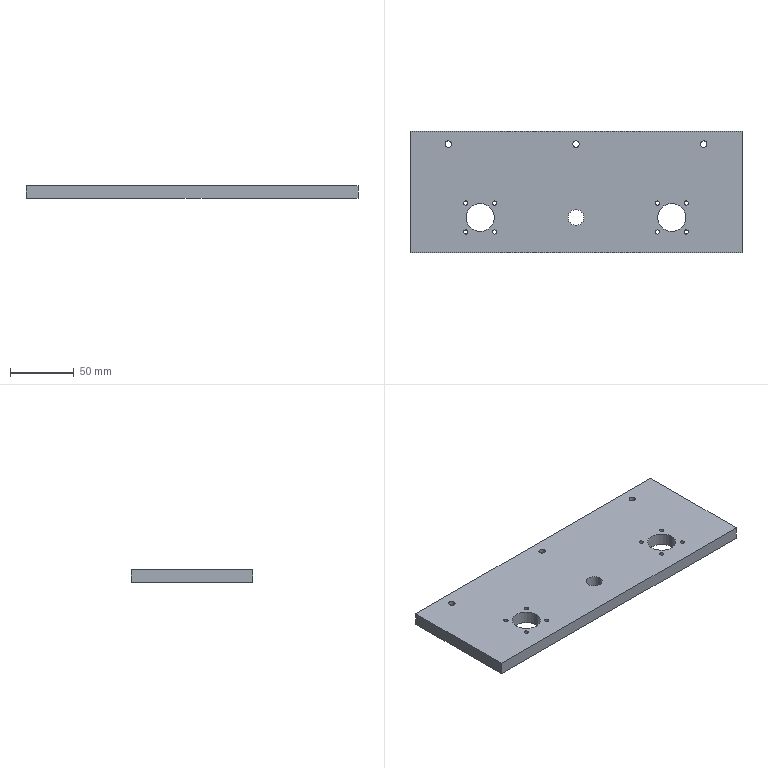Part | STEP file | X77-03201a | 1 solid | 34 faces | box 260 x 95 x 10 mm | volume 236897 mm3 | cylinder 28 | plane 6 | commonest cylinder face diameters 3.3 x16 5 x6 22 x4 12.5 x2
STEP:
#1=CARTESIAN_POINT('',(-98.5,85.,15.));
#2=VERTEX_POINT('',#1);
#3=CARTESIAN_POINT('',(-103.5,85.,15.));
#4=VERTEX_POINT('',#3);
#5=CARTESIAN_POINT('',(-101.,85.,15.));
#6=DIRECTION('',(0.,0.,-1.));
#7=DIRECTION('',(-1.,0.,0.));
#8=AXIS2_PLACEMENT_3D('',#5,#6,#7);
#9=CIRCLE('',#8,2.5);
#10=EDGE_CURVE('',#2,#4,#9,.T.);
#11=ORIENTED_EDGE('',*,*,#10,.F.);
#12=CARTESIAN_POINT('',(-98.5,85.,5.));
#13=VERTEX_POINT('',#12);
#14=CARTESIAN_POINT('',(-98.5,85.,5.));
#15=DIRECTION('',(0.,0.,-1.));
#16=VECTOR('',#15,1000.);
#17=LINE('',#14,#16);
#18=EDGE_CURVE('',#2,#13,#17,.T.);
#19=ORIENTED_EDGE('',*,*,#18,.T.);
#20=CARTESIAN_POINT('',(-103.5,85.,5.));
#21=VERTEX_POINT('',#20);
#22=CARTESIAN_POINT('',(-101.,85.,5.));
#23=DIRECTION('',(0.,0.,-1.));
#24=DIRECTION('',(-1.,0.,0.));
#25=AXIS2_PLACEMENT_3D('',#22,#23,#24);
#26=CIRCLE('',#25,2.5);
#27=EDGE_CURVE('',#13,#21,#26,.T.);
#28=ORIENTED_EDGE('',*,*,#27,.T.);
#29=CARTESIAN_POINT('',(-103.5,85.,5.));
#30=DIRECTION('',(0.,0.,-1.));
#31=VECTOR('',#30,1000.);
#32=LINE('',#29,#31);
#33=EDGE_CURVE('',#4,#21,#32,.T.);
#34=ORIENTED_EDGE('',*,*,#33,.F.);
#35=EDGE_LOOP('',(#11,#19,#28,#34));
#36=FACE_OUTER_BOUND('',#35,.T.);
#37=CARTESIAN_POINT('',(-101.,85.,5.));
#38=DIRECTION('',(0.,0.,-1.));
#39=DIRECTION('',(-1.,0.,0.));
#40=AXIS2_PLACEMENT_3D('',#37,#38,#39);
#41=CYLINDRICAL_SURFACE('',#40,2.5);
#42=ADVANCED_FACE('',(#36),#41,.F.);
#43=CARTESIAN_POINT('',(101.5,85.,15.));
#44=VERTEX_POINT('',#43);
#45=CARTESIAN_POINT('',(96.5,85.,15.));
#46=VERTEX_POINT('',#45);
#47=CARTESIAN_POINT('',(99.,85.,15.));
#48=DIRECTION('',(0.,0.,-1.));
#49=DIRECTION('',(-1.,0.,0.));
#50=AXIS2_PLACEMENT_3D('',#47,#48,#49);
#51=CIRCLE('',#50,2.5);
#52=EDGE_CURVE('',#44,#46,#51,.T.);
#53=ORIENTED_EDGE('',*,*,#52,.F.);
#54=CARTESIAN_POINT('',(101.5,85.,5.));
#55=VERTEX_POINT('',#54);
#56=CARTESIAN_POINT('',(101.5,85.,5.));
#57=DIRECTION('',(0.,0.,-1.));
#58=VECTOR('',#57,1000.);
#59=LINE('',#56,#58);
#60=EDGE_CURVE('',#44,#55,#59,.T.);
#61=ORIENTED_EDGE('',*,*,#60,.T.);
#62=CARTESIAN_POINT('',(96.5,85.,5.));
#63=VERTEX_POINT('',#62);
#64=CARTESIAN_POINT('',(99.,85.,5.));
#65=DIRECTION('',(0.,0.,-1.));
#66=DIRECTION('',(-1.,0.,0.));
#67=AXIS2_PLACEMENT_3D('',#64,#65,#66);
#68=CIRCLE('',#67,2.5);
#69=EDGE_CURVE('',#55,#63,#68,.T.);
#70=ORIENTED_EDGE('',*,*,#69,.T.);
#71=CARTESIAN_POINT('',(96.5,85.,5.));
#72=DIRECTION('',(0.,0.,-1.));
#73=VECTOR('',#72,1000.);
#74=LINE('',#71,#73);
#75=EDGE_CURVE('',#46,#63,#74,.T.);
#76=ORIENTED_EDGE('',*,*,#75,.F.);
#77=EDGE_LOOP('',(#53,#61,#70,#76));
#78=FACE_OUTER_BOUND('',#77,.T.);
#79=CARTESIAN_POINT('',(99.,85.,5.));
#80=DIRECTION('',(0.,0.,-1.));
#81=DIRECTION('',(-1.,0.,0.));
#82=AXIS2_PLACEMENT_3D('',#79,#80,#81);
#83=CYLINDRICAL_SURFACE('',#82,2.5);
#84=ADVANCED_FACE('',(#78),#83,.F.);
#85=CARTESIAN_POINT('',(1.5,85.,15.));
#86=VERTEX_POINT('',#85);
#87=CARTESIAN_POINT('',(-3.5,85.,15.));
#88=VERTEX_POINT('',#87);
#89=CARTESIAN_POINT('',(-1.,85.,15.));
#90=DIRECTION('',(0.,0.,-1.));
#91=DIRECTION('',(-1.,0.,0.));
#92=AXIS2_PLACEMENT_3D('',#89,#90,#91);
#93=CIRCLE('',#92,2.5);
#94=EDGE_CURVE('',#86,#88,#93,.T.);
#95=ORIENTED_EDGE('',*,*,#94,.F.);
#96=CARTESIAN_POINT('',(1.5,85.,5.));
#97=VERTEX_POINT('',#96);
#98=CARTESIAN_POINT('',(1.5,85.,5.));
#99=DIRECTION('',(0.,0.,-1.));
#100=VECTOR('',#99,1000.);
#101=LINE('',#98,#100);
#102=EDGE_CURVE('',#86,#97,#101,.T.);
#103=ORIENTED_EDGE('',*,*,#102,.T.);
#104=CARTESIAN_POINT('',(-3.5,85.,5.));
#105=VERTEX_POINT('',#104);
#106=CARTESIAN_POINT('',(-1.,85.,5.));
#107=DIRECTION('',(0.,0.,-1.));
#108=DIRECTION('',(-1.,0.,0.));
#109=AXIS2_PLACEMENT_3D('',#106,#107,#108);
#110=CIRCLE('',#109,2.5);
#111=EDGE_CURVE('',#97,#105,#110,.T.);
#112=ORIENTED_EDGE('',*,*,#111,.T.);
#113=CARTESIAN_POINT('',(-3.5,85.,5.));
#114=DIRECTION('',(0.,0.,-1.));
#115=VECTOR('',#114,1000.);
#116=LINE('',#113,#115);
#117=EDGE_CURVE('',#88,#105,#116,.T.);
#118=ORIENTED_EDGE('',*,*,#117,.F.);
#119=EDGE_LOOP('',(#95,#103,#112,#118));
#120=FACE_OUTER_BOUND('',#119,.T.);
#121=CARTESIAN_POINT('',(-1.,85.,5.));
#122=DIRECTION('',(0.,0.,-1.));
#123=DIRECTION('',(-1.,0.,0.));
#124=AXIS2_PLACEMENT_3D('',#121,#122,#123);
#125=CYLINDRICAL_SURFACE('',#124,2.5);
#126=ADVANCED_FACE('',(#120),#125,.F.);
#127=CARTESIAN_POINT('',(-65.,27.5,15.));
#128=VERTEX_POINT('',#127);
#129=CARTESIAN_POINT('',(-87.,27.5,15.));
#130=VERTEX_POINT('',#129);
#131=CARTESIAN_POINT('',(-76.,27.5,15.));
#132=DIRECTION('',(0.,0.,-1.));
#133=DIRECTION('',(-1.,0.,0.));
#134=AXIS2_PLACEMENT_3D('',#131,#132,#133);
#135=CIRCLE('',#134,11.);
#136=EDGE_CURVE('',#128,#130,#135,.T.);
#137=ORIENTED_EDGE('',*,*,#136,.F.);
#138=CARTESIAN_POINT('',(-65.,27.5,5.));
#139=VERTEX_POINT('',#138);
#140=CARTESIAN_POINT('',(-65.,27.5,15.));
#141=DIRECTION('',(0.,0.,-1.));
#142=VECTOR('',#141,1000.);
#143=LINE('',#140,#142);
#144=EDGE_CURVE('',#128,#139,#143,.T.);
#145=ORIENTED_EDGE('',*,*,#144,.T.);
#146=CARTESIAN_POINT('',(-87.,27.5,5.));
#147=VERTEX_POINT('',#146);
#148=CARTESIAN_POINT('',(-76.,27.5,5.));
#149=DIRECTION('',(0.,0.,-1.));
#150=DIRECTION('',(-1.,0.,0.));
#151=AXIS2_PLACEMENT_3D('',#148,#149,#150);
#152=CIRCLE('',#151,11.);
#153=EDGE_CURVE('',#139,#147,#152,.T.);
#154=ORIENTED_EDGE('',*,*,#153,.T.);
#155=CARTESIAN_POINT('',(-87.,27.5,15.));
#156=DIRECTION('',(0.,0.,-1.));
#157=VECTOR('',#156,1000.);
#158=LINE('',#155,#157);
#159=EDGE_CURVE('',#130,#147,#158,.T.);
#160=ORIENTED_EDGE('',*,*,#159,.F.);
#161=EDGE_LOOP('',(#137,#145,#154,#160));
#162=FACE_OUTER_BOUND('',#161,.T.);
#163=CARTESIAN_POINT('',(-76.,27.5,15.));
#164=DIRECTION('',(0.,0.,-1.));
#165=DIRECTION('',(-1.,0.,0.));
#166=AXIS2_PLACEMENT_3D('',#163,#164,#165);
#167=CYLINDRICAL_SURFACE('',#166,11.);
#168=ADVANCED_FACE('',(#162),#167,.F.);
#169=CARTESIAN_POINT('',(85.,27.5,15.));
#170=VERTEX_POINT('',#169);
#171=CARTESIAN_POINT('',(63.,27.5,15.));
#172=VERTEX_POINT('',#171);
#173=CARTESIAN_POINT('',(74.,27.5,15.));
#174=DIRECTION('',(0.,0.,-1.));
#175=DIRECTION('',(-1.,0.,0.));
#176=AXIS2_PLACEMENT_3D('',#173,#174,#175);
#177=CIRCLE('',#176,11.);
#178=EDGE_CURVE('',#170,#172,#177,.T.);
#179=ORIENTED_EDGE('',*,*,#178,.F.);
#180=CARTESIAN_POINT('',(85.,27.5,5.));
#181=VERTEX_POINT('',#180);
#182=CARTESIAN_POINT('',(85.,27.5,15.));
#183=DIRECTION('',(0.,0.,-1.));
#184=VECTOR('',#183,1000.);
#185=LINE('',#182,#184);
#186=EDGE_CURVE('',#170,#181,#185,.T.);
#187=ORIENTED_EDGE('',*,*,#186,.T.);
#188=CARTESIAN_POINT('',(63.,27.5,5.));
#189=VERTEX_POINT('',#188);
#190=CARTESIAN_POINT('',(74.,27.5,5.));
#191=DIRECTION('',(0.,0.,-1.));
#192=DIRECTION('',(-1.,0.,0.));
#193=AXIS2_PLACEMENT_3D('',#190,#191,#192);
#194=CIRCLE('',#193,11.);
#195=EDGE_CURVE('',#181,#189,#194,.T.);
#196=ORIENTED_EDGE('',*,*,#195,.T.);
#197=CARTESIAN_POINT('',(63.,27.5,15.));
#198=DIRECTION('',(0.,0.,-1.));
#199=VECTOR('',#198,1000.);
#200=LINE('',#197,#199);
#201=EDGE_CURVE('',#172,#189,#200,.T.);
#202=ORIENTED_EDGE('',*,*,#201,.F.);
#203=EDGE_LOOP('',(#179,#187,#196,#202));
#204=FACE_OUTER_BOUND('',#203,.T.);
#205=CARTESIAN_POINT('',(74.,27.5,15.));
#206=DIRECTION('',(0.,0.,-1.));
#207=DIRECTION('',(-1.,0.,0.));
#208=AXIS2_PLACEMENT_3D('',#205,#206,#207);
#209=CYLINDRICAL_SURFACE('',#208,11.);
#210=ADVANCED_FACE('',(#204),#209,.F.);
#211=CARTESIAN_POINT('',(-88.965,16.185,5.));
#212=VERTEX_POINT('',#211);
#213=CARTESIAN_POINT('',(-85.665,16.185,5.));
#214=VERTEX_POINT('',#213);
#215=CARTESIAN_POINT('',(-87.315,16.185,5.));
#216=DIRECTION('',(0.,0.,1.));
#217=DIRECTION('',(1.,0.,0.));
#218=AXIS2_PLACEMENT_3D('',#215,#216,#217);
#219=CIRCLE('',#218,1.65);
#220=EDGE_CURVE('',#212,#214,#219,.T.);
#221=ORIENTED_EDGE('',*,*,#220,.F.);
#222=CARTESIAN_POINT('',(-88.965,16.185,15.));
#223=VERTEX_POINT('',#222);
#224=CARTESIAN_POINT('',(-88.965,16.185,15.));
#225=DIRECTION('',(0.,0.,1.));
#226=VECTOR('',#225,1000.);
#227=LINE('',#224,#226);
#228=EDGE_CURVE('',#212,#223,#227,.T.);
#229=ORIENTED_EDGE('',*,*,#228,.T.);
#230=CARTESIAN_POINT('',(-85.665,16.185,15.));
#231=VERTEX_POINT('',#230);
#232=CARTESIAN_POINT('',(-87.315,16.185,15.));
#233=DIRECTION('',(0.,0.,1.));
#234=DIRECTION('',(1.,0.,0.));
#235=AXIS2_PLACEMENT_3D('',#232,#233,#234);
#236=CIRCLE('',#235,1.65);
#237=EDGE_CURVE('',#223,#231,#236,.T.);
#238=ORIENTED_EDGE('',*,*,#237,.T.);
#239=CARTESIAN_POINT('',(-85.665,16.185,15.));
#240=DIRECTION('',(0.,0.,1.));
#241=VECTOR('',#240,1000.);
#242=LINE('',#239,#241);
#243=EDGE_CURVE('',#214,#231,#242,.T.);
#244=ORIENTED_EDGE('',*,*,#243,.F.);
#245=EDGE_LOOP('',(#221,#229,#238,#244));
#246=FACE_OUTER_BOUND('',#245,.T.);
#247=CARTESIAN_POINT('',(-87.315,16.185,15.));
#248=DIRECTION('',(0.,0.,1.));
#249=DIRECTION('',(1.,0.,0.));
#250=AXIS2_PLACEMENT_3D('',#247,#248,#249);
#251=CYLINDRICAL_SURFACE('',#250,1.65);
#252=ADVANCED_FACE('',(#246),#251,.F.);
#253=CARTESIAN_POINT('',(-66.338,16.188,5.));
#254=VERTEX_POINT('',#253);
#255=CARTESIAN_POINT('',(-63.038,16.188,5.));
#256=VERTEX_POINT('',#255);
#257=CARTESIAN_POINT('',(-64.688,16.188,5.));
#258=DIRECTION('',(0.,0.,1.));
#259=DIRECTION('',(1.,0.,0.));
#260=AXIS2_PLACEMENT_3D('',#257,#258,#259);
#261=CIRCLE('',#260,1.65);
#262=EDGE_CURVE('',#254,#256,#261,.T.);
#263=ORIENTED_EDGE('',*,*,#262,.F.);
#264=CARTESIAN_POINT('',(-66.338,16.188,15.));
#265=VERTEX_POINT('',#264);
#266=CARTESIAN_POINT('',(-66.338,16.188,15.));
#267=DIRECTION('',(0.,0.,1.));
#268=VECTOR('',#267,1000.);
#269=LINE('',#266,#268);
#270=EDGE_CURVE('',#254,#265,#269,.T.);
#271=ORIENTED_EDGE('',*,*,#270,.T.);
#272=CARTESIAN_POINT('',(-63.038,16.188,15.));
#273=VERTEX_POINT('',#272);
#274=CARTESIAN_POINT('',(-64.688,16.188,15.));
#275=DIRECTION('',(0.,0.,1.));
#276=DIRECTION('',(1.,0.,0.));
#277=AXIS2_PLACEMENT_3D('',#274,#275,#276);
#278=CIRCLE('',#277,1.65);
#279=EDGE_CURVE('',#265,#273,#278,.T.);
#280=ORIENTED_EDGE('',*,*,#279,.T.);
#281=CARTESIAN_POINT('',(-63.038,16.188,15.));
#282=DIRECTION('',(0.,0.,1.));
#283=VECTOR('',#282,1000.);
#284=LINE('',#281,#283);
#285=EDGE_CURVE('',#256,#273,#284,.T.);
#286=ORIENTED_EDGE('',*,*,#285,.F.);
#287=EDGE_LOOP('',(#263,#271,#280,#286));
#288=FACE_OUTER_BOUND('',#287,.T.);
#289=CARTESIAN_POINT('',(-64.688,16.188,15.));
#290=DIRECTION('',(0.,0.,1.));
#291=DIRECTION('',(1.,0.,0.));
#292=AXIS2_PLACEMENT_3D('',#289,#290,#291);
#293=CYLINDRICAL_SURFACE('',#292,1.65);
#294=ADVANCED_FACE('',(#288),#293,.F.);
#295=CARTESIAN_POINT('',(-66.335,38.815,5.));
#296=VERTEX_POINT('',#295);
#297=CARTESIAN_POINT('',(-63.035,38.815,5.));
#298=VERTEX_POINT('',#297);
#299=CARTESIAN_POINT('',(-64.685,38.815,5.));
#300=DIRECTION('',(0.,0.,1.));
#301=DIRECTION('',(1.,0.,0.));
#302=AXIS2_PLACEMENT_3D('',#299,#300,#301);
#303=CIRCLE('',#302,1.65);
#304=EDGE_CURVE('',#296,#298,#303,.T.);
#305=ORIENTED_EDGE('',*,*,#304,.F.);
#306=CARTESIAN_POINT('',(-66.335,38.815,15.));
#307=VERTEX_POINT('',#306);
#308=CARTESIAN_POINT('',(-66.335,38.815,15.));
#309=DIRECTION('',(0.,0.,1.));
#310=VECTOR('',#309,1000.);
#311=LINE('',#308,#310);
#312=EDGE_CURVE('',#296,#307,#311,.T.);
#313=ORIENTED_EDGE('',*,*,#312,.T.);
#314=CARTESIAN_POINT('',(-63.035,38.815,15.));
#315=VERTEX_POINT('',#314);
#316=CARTESIAN_POINT('',(-64.685,38.815,15.));
#317=DIRECTION('',(0.,0.,1.));
#318=DIRECTION('',(1.,0.,0.));
#319=AXIS2_PLACEMENT_3D('',#316,#317,#318);
#320=CIRCLE('',#319,1.65);
#321=EDGE_CURVE('',#307,#315,#320,.T.);
#322=ORIENTED_EDGE('',*,*,#321,.T.);
#323=CARTESIAN_POINT('',(-63.035,38.815,15.));
#324=DIRECTION('',(0.,0.,1.));
#325=VECTOR('',#324,1000.);
#326=LINE('',#323,#325);
#327=EDGE_CURVE('',#298,#315,#326,.T.);
#328=ORIENTED_EDGE('',*,*,#327,.F.);
#329=EDGE_LOOP('',(#305,#313,#322,#328));
#330=FACE_OUTER_BOUND('',#329,.T.);
#331=CARTESIAN_POINT('',(-64.685,38.815,15.));
#332=DIRECTION('',(0.,0.,1.));
#333=DIRECTION('',(1.,0.,0.));
#334=AXIS2_PLACEMENT_3D('',#331,#332,#333);
#335=CYLINDRICAL_SURFACE('',#334,1.65);
#336=ADVANCED_FACE('',(#330),#335,.F.);
#337=CARTESIAN_POINT('',(-88.965,38.815,5.));
#338=VERTEX_POINT('',#337);
#339=CARTESIAN_POINT('',(-85.665,38.815,5.));
#340=VERTEX_POINT('',#339);
#341=CARTESIAN_POINT('',(-87.315,38.815,5.));
#342=DIRECTION('',(0.,0.,1.));
#343=DIRECTION('',(1.,0.,0.));
#344=AXIS2_PLACEMENT_3D('',#341,#342,#343);
#345=CIRCLE('',#344,1.65);
#346=EDGE_CURVE('',#338,#340,#345,.T.);
#347=ORIENTED_EDGE('',*,*,#346,.F.);
#348=CARTESIAN_POINT('',(-88.965,38.815,15.));
#349=VERTEX_POINT('',#348);
#350=CARTESIAN_POINT('',(-88.965,38.815,15.));
#351=DIRECTION('',(0.,0.,1.));
#352=VECTOR('',#351,1000.);
#353=LINE('',#350,#352);
#354=EDGE_CURVE('',#338,#349,#353,.T.);
#355=ORIENTED_EDGE('',*,*,#354,.T.);
#356=CARTESIAN_POINT('',(-85.665,38.815,15.));
#357=VERTEX_POINT('',#356);
#358=CARTESIAN_POINT('',(-87.315,38.815,15.));
#359=DIRECTION('',(0.,0.,1.));
#360=DIRECTION('',(1.,0.,0.));
#361=AXIS2_PLACEMENT_3D('',#358,#359,#360);
#362=CIRCLE('',#361,1.65);
#363=EDGE_CURVE('',#349,#357,#362,.T.);
#364=ORIENTED_EDGE('',*,*,#363,.T.);
#365=CARTESIAN_POINT('',(-85.665,38.815,15.));
#366=DIRECTION('',(0.,0.,1.));
#367=VECTOR('',#366,1000.);
#368=LINE('',#365,#367);
#369=EDGE_CURVE('',#340,#357,#368,.T.);
#370=ORIENTED_EDGE('',*,*,#369,.F.);
#371=EDGE_LOOP('',(#347,#355,#364,#370));
#372=FACE_OUTER_BOUND('',#371,.T.);
#373=CARTESIAN_POINT('',(-87.315,38.815,15.));
#374=DIRECTION('',(0.,0.,1.));
#375=DIRECTION('',(1.,0.,0.));
#376=AXIS2_PLACEMENT_3D('',#373,#374,#375);
#377=CYLINDRICAL_SURFACE('',#376,1.65);
#378=ADVANCED_FACE('',(#372),#377,.F.);
#379=CARTESIAN_POINT('',(61.038,16.188,5.));
#380=VERTEX_POINT('',#379);
#381=CARTESIAN_POINT('',(64.338,16.188,5.));
#382=VERTEX_POINT('',#381);
#383=CARTESIAN_POINT('',(62.688,16.188,5.));
#384=DIRECTION('',(0.,0.,1.));
#385=DIRECTION('',(1.,0.,0.));
#386=AXIS2_PLACEMENT_3D('',#383,#384,#385);
#387=CIRCLE('',#386,1.65);
#388=EDGE_CURVE('',#380,#382,#387,.T.);
#389=ORIENTED_EDGE('',*,*,#388,.F.);
#390=CARTESIAN_POINT('',(61.038,16.188,15.));
#391=VERTEX_POINT('',#390);
#392=CARTESIAN_POINT('',(61.038,16.188,15.));
#393=DIRECTION('',(0.,0.,1.));
#394=VECTOR('',#393,1000.);
#395=LINE('',#392,#394);
#396=EDGE_CURVE('',#380,#391,#395,.T.);
#397=ORIENTED_EDGE('',*,*,#396,.T.);
#398=CARTESIAN_POINT('',(64.338,16.188,15.));
#399=VERTEX_POINT('',#398);
#400=CARTESIAN_POINT('',(62.688,16.188,15.));
#401=DIRECTION('',(0.,0.,1.));
#402=DIRECTION('',(1.,0.,0.));
#403=AXIS2_PLACEMENT_3D('',#400,#401,#402);
#404=CIRCLE('',#403,1.65);
#405=EDGE_CURVE('',#391,#399,#404,.T.);
#406=ORIENTED_EDGE('',*,*,#405,.T.);
#407=CARTESIAN_POINT('',(64.338,16.188,15.));
#408=DIRECTION('',(0.,0.,1.));
#409=VECTOR('',#408,1000.);
#410=LINE('',#407,#409);
#411=EDGE_CURVE('',#382,#399,#410,.T.);
#412=ORIENTED_EDGE('',*,*,#411,.F.);
#413=EDGE_LOOP('',(#389,#397,#406,#412));
#414=FACE_OUTER_BOUND('',#413,.T.);
#415=CARTESIAN_POINT('',(62.688,16.188,15.));
#416=DIRECTION('',(0.,0.,1.));
#417=DIRECTION('',(1.,0.,0.));
#418=AXIS2_PLACEMENT_3D('',#415,#416,#417);
#419=CYLINDRICAL_SURFACE('',#418,1.65);
#420=ADVANCED_FACE('',(#414),#419,.F.);
#421=CARTESIAN_POINT('',(83.665,16.185,5.));
#422=VERTEX_POINT('',#421);
#423=CARTESIAN_POINT('',(86.965,16.185,5.));
#424=VERTEX_POINT('',#423);
#425=CARTESIAN_POINT('',(85.315,16.185,5.));
#426=DIRECTION('',(0.,0.,1.));
#427=DIRECTION('',(1.,0.,0.));
#428=AXIS2_PLACEMENT_3D('',#425,#426,#427);
#429=CIRCLE('',#428,1.65);
#430=EDGE_CURVE('',#422,#424,#429,.T.);
#431=ORIENTED_EDGE('',*,*,#430,.F.);
#432=CARTESIAN_POINT('',(83.665,16.185,15.));
#433=VERTEX_POINT('',#432);
#434=CARTESIAN_POINT('',(83.665,16.185,15.));
#435=DIRECTION('',(0.,0.,1.));
#436=VECTOR('',#435,1000.);
#437=LINE('',#434,#436);
#438=EDGE_CURVE('',#422,#433,#437,.T.);
#439=ORIENTED_EDGE('',*,*,#438,.T.);
#440=CARTESIAN_POINT('',(86.965,16.185,15.));
#441=VERTEX_POINT('',#440);
#442=CARTESIAN_POINT('',(85.315,16.185,15.));
#443=DIRECTION('',(0.,0.,1.));
#444=DIRECTION('',(1.,0.,0.));
#445=AXIS2_PLACEMENT_3D('',#442,#443,#444);
#446=CIRCLE('',#445,1.65);
#447=EDGE_CURVE('',#433,#441,#446,.T.);
#448=ORIENTED_EDGE('',*,*,#447,.T.);
#449=CARTESIAN_POINT('',(86.965,16.185,15.));
#450=DIRECTION('',(0.,0.,1.));
#451=VECTOR('',#450,1000.);
#452=LINE('',#449,#451);
#453=EDGE_CURVE('',#424,#441,#452,.T.);
#454=ORIENTED_EDGE('',*,*,#453,.F.);
#455=EDGE_LOOP('',(#431,#439,#448,#454));
#456=FACE_OUTER_BOUND('',#455,.T.);
#457=CARTESIAN_POINT('',(85.315,16.185,15.));
#458=DIRECTION('',(0.,0.,1.));
#459=DIRECTION('',(1.,0.,0.));
#460=AXIS2_PLACEMENT_3D('',#457,#458,#459);
#461=CYLINDRICAL_SURFACE('',#460,1.65);
#462=ADVANCED_FACE('',(#456),#461,.F.);
#463=CARTESIAN_POINT('',(61.035,38.815,5.));
#464=VERTEX_POINT('',#463);
#465=CARTESIAN_POINT('',(64.335,38.815,5.));
#466=VERTEX_POINT('',#465);
#467=CARTESIAN_POINT('',(62.685,38.815,5.));
#468=DIRECTION('',(0.,0.,1.));
#469=DIRECTION('',(1.,0.,0.));
#470=AXIS2_PLACEMENT_3D('',#467,#468,#469);
#471=CIRCLE('',#470,1.65);
#472=EDGE_CURVE('',#464,#466,#471,.T.);
#473=ORIENTED_EDGE('',*,*,#472,.F.);
#474=CARTESIAN_POINT('',(61.035,38.815,15.));
#475=VERTEX_POINT('',#474);
#476=CARTESIAN_POINT('',(61.035,38.815,15.));
#477=DIRECTION('',(0.,0.,1.));
#478=VECTOR('',#477,1000.);
#479=LINE('',#476,#478);
#480=EDGE_CURVE('',#464,#475,#479,.T.);
#481=ORIENTED_EDGE('',*,*,#480,.T.);
#482=CARTESIAN_POINT('',(64.335,38.815,15.));
#483=VERTEX_POINT('',#482);
#484=CARTESIAN_POINT('',(62.685,38.815,15.));
#485=DIRECTION('',(0.,0.,1.));
#486=DIRECTION('',(1.,0.,0.));
#487=AXIS2_PLACEMENT_3D('',#484,#485,#486);
#488=CIRCLE('',#487,1.65);
#489=EDGE_CURVE('',#475,#483,#488,.T.);
#490=ORIENTED_EDGE('',*,*,#489,.T.);
#491=CARTESIAN_POINT('',(64.335,38.815,15.));
#492=DIRECTION('',(0.,0.,1.));
#493=VECTOR('',#492,1000.);
#494=LINE('',#491,#493);
#495=EDGE_CURVE('',#466,#483,#494,.T.);
#496=ORIENTED_EDGE('',*,*,#495,.F.);
#497=EDGE_LOOP('',(#473,#481,#490,#496));
#498=FACE_OUTER_BOUND('',#497,.T.);
#499=CARTESIAN_POINT('',(62.685,38.815,15.));
#500=DIRECTION('',(0.,0.,1.));
#501=DIRECTION('',(1.,0.,0.));
#502=AXIS2_PLACEMENT_3D('',#499,#500,#501);
#503=CYLINDRICAL_SURFACE('',#502,1.65);
#504=ADVANCED_FACE('',(#498),#503,.F.);
#505=CARTESIAN_POINT('',(83.665,38.815,5.));
#506=VERTEX_POINT('',#505);
#507=CARTESIAN_POINT('',(86.965,38.815,5.));
#508=VERTEX_POINT('',#507);
#509=CARTESIAN_POINT('',(85.315,38.815,5.));
#510=DIRECTION('',(0.,0.,1.));
#511=DIRECTION('',(1.,0.,0.));
#512=AXIS2_PLACEMENT_3D('',#509,#510,#511);
#513=CIRCLE('',#512,1.65);
#514=EDGE_CURVE('',#506,#508,#513,.T.);
#515=ORIENTED_EDGE('',*,*,#514,.F.);
#516=CARTESIAN_POINT('',(83.665,38.815,15.));
#517=VERTEX_POINT('',#516);
#518=CARTESIAN_POINT('',(83.665,38.815,15.));
#519=DIRECTION('',(0.,0.,1.));
#520=VECTOR('',#519,1000.);
#521=LINE('',#518,#520);
#522=EDGE_CURVE('',#506,#517,#521,.T.);
#523=ORIENTED_EDGE('',*,*,#522,.T.);
#524=CARTESIAN_POINT('',(86.965,38.815,15.));
#525=VERTEX_POINT('',#524);
#526=CARTESIAN_POINT('',(85.315,38.815,15.));
#527=DIRECTION('',(0.,0.,1.));
#528=DIRECTION('',(1.,0.,0.));
#529=AXIS2_PLACEMENT_3D('',#526,#527,#528);
#530=CIRCLE('',#529,1.65);
#531=EDGE_CURVE('',#517,#525,#530,.T.);
#532=ORIENTED_EDGE('',*,*,#531,.T.);
#533=CARTESIAN_POINT('',(86.965,38.815,15.));
#534=DIRECTION('',(0.,0.,1.));
#535=VECTOR('',#534,1000.);
#536=LINE('',#533,#535);
#537=EDGE_CURVE('',#508,#525,#536,.T.);
#538=ORIENTED_EDGE('',*,*,#537,.F.);
#539=EDGE_LOOP('',(#515,#523,#532,#538));
#540=FACE_OUTER_BOUND('',#539,.T.);
#541=CARTESIAN_POINT('',(85.315,38.815,15.));
#542=DIRECTION('',(0.,0.,1.));
#543=DIRECTION('',(1.,0.,0.));
#544=AXIS2_PLACEMENT_3D('',#541,#542,#543);
#545=CYLINDRICAL_SURFACE('',#544,1.65);
#546=ADVANCED_FACE('',(#540),#545,.F.);
#547=CARTESIAN_POINT('',(-7.25,27.5,5.));
#548=VERTEX_POINT('',#547);
#549=CARTESIAN_POINT('',(5.25,27.5,5.));
#550=VERTEX_POINT('',#549);
#551=CARTESIAN_POINT('',(-1.,27.5,5.));
#552=DIRECTION('',(0.,0.,1.));
#553=DIRECTION('',(1.,0.,0.));
#554=AXIS2_PLACEMENT_3D('',#551,#552,#553);
#555=CIRCLE('',#554,6.25);
#556=EDGE_CURVE('',#548,#550,#555,.T.);
#557=ORIENTED_EDGE('',*,*,#556,.F.);
#558=CARTESIAN_POINT('',(-7.25,27.5,15.));
#559=VERTEX_POINT('',#558);
#560=CARTESIAN_POINT('',(-7.25,27.5,15.));
#561=DIRECTION('',(0.,0.,1.));
#562=VECTOR('',#561,1000.);
#563=LINE('',#560,#562);
#564=EDGE_CURVE('',#548,#559,#563,.T.);
#565=ORIENTED_EDGE('',*,*,#564,.T.);
#566=CARTESIAN_POINT('',(5.25,27.5,15.));
#567=VERTEX_POINT('',#566);
#568=CARTESIAN_POINT('',(-1.,27.5,15.));
#569=DIRECTION('',(0.,0.,1.));
#570=DIRECTION('',(1.,0.,0.));
#571=AXIS2_PLACEMENT_3D('',#568,#569,#570);
#572=CIRCLE('',#571,6.25);
#573=EDGE_CURVE('',#559,#567,#572,.T.);
#574=ORIENTED_EDGE('',*,*,#573,.T.);
#575=CARTESIAN_POINT('',(5.25,27.5,15.));
#576=DIRECTION('',(0.,0.,1.));
#577=VECTOR('',#576,1000.);
#578=LINE('',#575,#577);
#579=EDGE_CURVE('',#550,#567,#578,.T.);
#580=ORIENTED_EDGE('',*,*,#579,.F.);
#581=EDGE_LOOP('',(#557,#565,#574,#580));
#582=FACE_OUTER_BOUND('',#581,.T.);
#583=CARTESIAN_POINT('',(-1.,27.5,15.));
#584=DIRECTION('',(0.,0.,1.));
#585=DIRECTION('',(1.,0.,0.));
#586=AXIS2_PLACEMENT_3D('',#583,#584,#585);
#587=CYLINDRICAL_SURFACE('',#586,6.25);
#588=ADVANCED_FACE('',(#582),#587,.F.);
#589=CARTESIAN_POINT('',(-101.,85.,5.));
#590=DIRECTION('',(0.,0.,-1.));
#591=DIRECTION('',(-1.,0.,0.));
#592=AXIS2_PLACEMENT_3D('',#589,#590,#591);
#593=CIRCLE('',#592,2.5);
#594=EDGE_CURVE('',#21,#13,#593,.T.);
#595=ORIENTED_EDGE('',*,*,#594,.F.);
#596=ORIENTED_EDGE('',*,*,#27,.F.);
#597=EDGE_LOOP('',(#595,#596));
#598=FACE_BOUND('',#597,.T.);
#599=CARTESIAN_POINT('',(99.,85.,5.));
#600=DIRECTION('',(0.,0.,-1.));
#601=DIRECTION('',(-1.,0.,0.));
#602=AXIS2_PLACEMENT_3D('',#599,#600,#601);
#603=CIRCLE('',#602,2.5);
#604=EDGE_CURVE('',#63,#55,#603,.T.);
#605=ORIENTED_EDGE('',*,*,#604,.F.);
#606=ORIENTED_EDGE('',*,*,#69,.F.);
#607=EDGE_LOOP('',(#605,#606));
#608=FACE_BOUND('',#607,.T.);
#609=CARTESIAN_POINT('',(-1.,85.,5.));
#610=DIRECTION('',(0.,0.,-1.));
#611=DIRECTION('',(-1.,0.,0.));
#612=AXIS2_PLACEMENT_3D('',#609,#610,#611);
#613=CIRCLE('',#612,2.5);
#614=EDGE_CURVE('',#105,#97,#613,.T.);
#615=ORIENTED_EDGE('',*,*,#614,.F.);
#616=ORIENTED_EDGE('',*,*,#111,.F.);
#617=EDGE_LOOP('',(#615,#616));
#618=FACE_BOUND('',#617,.T.);
#619=CARTESIAN_POINT('',(-76.,27.5,5.));
#620=DIRECTION('',(0.,0.,-1.));
#621=DIRECTION('',(-1.,0.,0.));
#622=AXIS2_PLACEMENT_3D('',#619,#620,#621);
#623=CIRCLE('',#622,11.);
#624=EDGE_CURVE('',#147,#139,#623,.T.);
#625=ORIENTED_EDGE('',*,*,#624,.F.);
#626=ORIENTED_EDGE('',*,*,#153,.F.);
#627=EDGE_LOOP('',(#625,#626));
#628=FACE_BOUND('',#627,.T.);
#629=CARTESIAN_POINT('',(74.,27.5,5.));
#630=DIRECTION('',(0.,0.,-1.));
#631=DIRECTION('',(-1.,0.,0.));
#632=AXIS2_PLACEMENT_3D('',#629,#630,#631);
#633=CIRCLE('',#632,11.);
#634=EDGE_CURVE('',#189,#181,#633,.T.);
#635=ORIENTED_EDGE('',*,*,#634,.F.);
#636=ORIENTED_EDGE('',*,*,#195,.F.);
#637=EDGE_LOOP('',(#635,#636));
#638=FACE_BOUND('',#637,.T.);
#639=CARTESIAN_POINT('',(-87.315,16.185,5.));
#640=DIRECTION('',(0.,0.,1.));
#641=DIRECTION('',(1.,0.,0.));
#642=AXIS2_PLACEMENT_3D('',#639,#640,#641);
#643=CIRCLE('',#642,1.65);
#644=EDGE_CURVE('',#214,#212,#643,.T.);
#645=ORIENTED_EDGE('',*,*,#644,.T.);
#646=ORIENTED_EDGE('',*,*,#220,.T.);
#647=EDGE_LOOP('',(#645,#646));
#648=FACE_BOUND('',#647,.T.);
#649=CARTESIAN_POINT('',(-64.688,16.188,5.));
#650=DIRECTION('',(0.,0.,1.));
#651=DIRECTION('',(1.,0.,0.));
#652=AXIS2_PLACEMENT_3D('',#649,#650,#651);
#653=CIRCLE('',#652,1.65);
#654=EDGE_CURVE('',#256,#254,#653,.T.);
#655=ORIENTED_EDGE('',*,*,#654,.T.);
#656=ORIENTED_EDGE('',*,*,#262,.T.);
#657=EDGE_LOOP('',(#655,#656));
#658=FACE_BOUND('',#657,.T.);
#659=CARTESIAN_POINT('',(-64.685,38.815,5.));
#660=DIRECTION('',(0.,0.,1.));
#661=DIRECTION('',(1.,0.,0.));
#662=AXIS2_PLACEMENT_3D('',#659,#660,#661);
#663=CIRCLE('',#662,1.65);
#664=EDGE_CURVE('',#298,#296,#663,.T.);
#665=ORIENTED_EDGE('',*,*,#664,.T.);
#666=ORIENTED_EDGE('',*,*,#304,.T.);
#667=EDGE_LOOP('',(#665,#666));
#668=FACE_BOUND('',#667,.T.);
#669=CARTESIAN_POINT('',(-87.315,38.815,5.));
#670=DIRECTION('',(0.,0.,1.));
#671=DIRECTION('',(1.,0.,0.));
#672=AXIS2_PLACEMENT_3D('',#669,#670,#671);
#673=CIRCLE('',#672,1.65);
#674=EDGE_CURVE('',#340,#338,#673,.T.);
#675=ORIENTED_EDGE('',*,*,#674,.T.);
#676=ORIENTED_EDGE('',*,*,#346,.T.);
#677=EDGE_LOOP('',(#675,#676));
#678=FACE_BOUND('',#677,.T.);
#679=CARTESIAN_POINT('',(62.688,16.188,5.));
#680=DIRECTION('',(0.,0.,1.));
#681=DIRECTION('',(1.,0.,0.));
#682=AXIS2_PLACEMENT_3D('',#679,#680,#681);
#683=CIRCLE('',#682,1.65);
#684=EDGE_CURVE('',#382,#380,#683,.T.);
#685=ORIENTED_EDGE('',*,*,#684,.T.);
#686=ORIENTED_EDGE('',*,*,#388,.T.);
#687=EDGE_LOOP('',(#685,#686));
#688=FACE_BOUND('',#687,.T.);
#689=CARTESIAN_POINT('',(85.315,16.185,5.));
#690=DIRECTION('',(0.,0.,1.));
#691=DIRECTION('',(1.,0.,0.));
#692=AXIS2_PLACEMENT_3D('',#689,#690,#691);
#693=CIRCLE('',#692,1.65);
#694=EDGE_CURVE('',#424,#422,#693,.T.);
#695=ORIENTED_EDGE('',*,*,#694,.T.);
#696=ORIENTED_EDGE('',*,*,#430,.T.);
#697=EDGE_LOOP('',(#695,#696));
#698=FACE_BOUND('',#697,.T.);
#699=CARTESIAN_POINT('',(62.685,38.815,5.));
#700=DIRECTION('',(0.,0.,1.));
#701=DIRECTION('',(1.,0.,0.));
#702=AXIS2_PLACEMENT_3D('',#699,#700,#701);
#703=CIRCLE('',#702,1.65);
#704=EDGE_CURVE('',#466,#464,#703,.T.);
#705=ORIENTED_EDGE('',*,*,#704,.T.);
#706=ORIENTED_EDGE('',*,*,#472,.T.);
#707=EDGE_LOOP('',(#705,#706));
#708=FACE_BOUND('',#707,.T.);
#709=CARTESIAN_POINT('',(85.315,38.815,5.));
#710=DIRECTION('',(0.,0.,1.));
#711=DIRECTION('',(1.,0.,0.));
#712=AXIS2_PLACEMENT_3D('',#709,#710,#711);
#713=CIRCLE('',#712,1.65);
#714=EDGE_CURVE('',#508,#506,#713,.T.);
#715=ORIENTED_EDGE('',*,*,#714,.T.);
#716=ORIENTED_EDGE('',*,*,#514,.T.);
#717=EDGE_LOOP('',(#715,#716));
#718=FACE_BOUND('',#717,.T.);
#719=CARTESIAN_POINT('',(-1.,27.5,5.));
#720=DIRECTION('',(0.,0.,1.));
#721=DIRECTION('',(1.,0.,0.));
#722=AXIS2_PLACEMENT_3D('',#719,#720,#721);
#723=CIRCLE('',#722,6.25);
#724=EDGE_CURVE('',#550,#548,#723,.T.);
#725=ORIENTED_EDGE('',*,*,#724,.T.);
#726=ORIENTED_EDGE('',*,*,#556,.T.);
#727=EDGE_LOOP('',(#725,#726));
#728=FACE_BOUND('',#727,.T.);
#729=CARTESIAN_POINT('',(129.,0.,5.));
#730=VERTEX_POINT('',#729);
#731=CARTESIAN_POINT('',(-131.,0.,5.));
#732=VERTEX_POINT('',#731);
#733=CARTESIAN_POINT('',(-131.,0.,5.));
#734=DIRECTION('',(-1.,0.,0.));
#735=VECTOR('',#734,1000.);
#736=LINE('',#733,#735);
#737=EDGE_CURVE('',#730,#732,#736,.T.);
#738=ORIENTED_EDGE('',*,*,#737,.T.);
#739=CARTESIAN_POINT('',(-131.,95.,5.));
#740=VERTEX_POINT('',#739);
#741=CARTESIAN_POINT('',(-131.,55.,5.));
#742=DIRECTION('',(0.,-1.,0.));
#743=VECTOR('',#742,1000.);
#744=LINE('',#741,#743);
#745=EDGE_CURVE('',#740,#732,#744,.T.);
#746=ORIENTED_EDGE('',*,*,#745,.F.);
#747=CARTESIAN_POINT('',(129.,95.,5.));
#748=VERTEX_POINT('',#747);
#749=CARTESIAN_POINT('',(129.,95.,5.));
#750=DIRECTION('',(-1.,0.,0.));
#751=VECTOR('',#750,1000.);
#752=LINE('',#749,#751);
#753=EDGE_CURVE('',#748,#740,#752,.T.);
#754=ORIENTED_EDGE('',*,*,#753,.F.);
#755=CARTESIAN_POINT('',(129.,55.,5.));
#756=DIRECTION('',(0.,-1.,0.));
#757=VECTOR('',#756,1000.);
#758=LINE('',#755,#757);
#759=EDGE_CURVE('',#748,#730,#758,.T.);
#760=ORIENTED_EDGE('',*,*,#759,.T.);
#761=EDGE_LOOP('',(#738,#746,#754,#760));
#762=FACE_OUTER_BOUND('',#761,.T.);
#763=CARTESIAN_POINT('',(-131.,55.,5.));
#764=DIRECTION('',(0.,0.,1.));
#765=DIRECTION('',(1.,0.,0.));
#766=AXIS2_PLACEMENT_3D('',#763,#764,#765);
#767=PLANE('',#766);
#768=ADVANCED_FACE('',(#598,#608,#618,#628,#638,#648,#658,#668,#678,#688,#698,#708,#718,#728,#762),#767,.F.);
#769=CARTESIAN_POINT('',(-131.,0.,15.));
#770=VERTEX_POINT('',#769);
#771=CARTESIAN_POINT('',(-131.,0.,5.));
#772=DIRECTION('',(0.,0.,1.));
#773=VECTOR('',#772,1000.);
#774=LINE('',#771,#773);
#775=EDGE_CURVE('',#732,#770,#774,.T.);
#776=ORIENTED_EDGE('',*,*,#775,.T.);
#777=CARTESIAN_POINT('',(-131.,95.,15.));
#778=VERTEX_POINT('',#777);
#779=CARTESIAN_POINT('',(-131.,55.,15.));
#780=DIRECTION('',(0.,-1.,0.));
#781=VECTOR('',#780,1000.);
#782=LINE('',#779,#781);
#783=EDGE_CURVE('',#778,#770,#782,.T.);
#784=ORIENTED_EDGE('',*,*,#783,.F.);
#785=CARTESIAN_POINT('',(-131.,95.,5.));
#786=DIRECTION('',(0.,0.,1.));
#787=VECTOR('',#786,1000.);
#788=LINE('',#785,#787);
#789=EDGE_CURVE('',#740,#778,#788,.T.);
#790=ORIENTED_EDGE('',*,*,#789,.F.);
#791=ORIENTED_EDGE('',*,*,#745,.T.);
#792=EDGE_LOOP('',(#776,#784,#790,#791));
#793=FACE_OUTER_BOUND('',#792,.T.);
#794=CARTESIAN_POINT('',(-131.,55.,5.));
#795=DIRECTION('',(1.,0.,0.));
#796=DIRECTION('',(0.,0.,-1.));
#797=AXIS2_PLACEMENT_3D('',#794,#795,#796);
#798=PLANE('',#797);
#799=ADVANCED_FACE('',(#793),#798,.F.);
#800=CARTESIAN_POINT('',(-101.,85.,15.));
#801=DIRECTION('',(0.,0.,-1.));
#802=DIRECTION('',(-1.,0.,0.));
#803=AXIS2_PLACEMENT_3D('',#800,#801,#802);
#804=CIRCLE('',#803,2.5);
#805=EDGE_CURVE('',#4,#2,#804,.T.);
#806=ORIENTED_EDGE('',*,*,#805,.T.);
#807=ORIENTED_EDGE('',*,*,#10,.T.);
#808=EDGE_LOOP('',(#806,#807));
#809=FACE_BOUND('',#808,.T.);
#810=CARTESIAN_POINT('',(99.,85.,15.));
#811=DIRECTION('',(0.,0.,-1.));
#812=DIRECTION('',(-1.,0.,0.));
#813=AXIS2_PLACEMENT_3D('',#810,#811,#812);
#814=CIRCLE('',#813,2.5);
#815=EDGE_CURVE('',#46,#44,#814,.T.);
#816=ORIENTED_EDGE('',*,*,#815,.T.);
#817=ORIENTED_EDGE('',*,*,#52,.T.);
#818=EDGE_LOOP('',(#816,#817));
#819=FACE_BOUND('',#818,.T.);
#820=CARTESIAN_POINT('',(-1.,85.,15.));
#821=DIRECTION('',(0.,0.,-1.));
#822=DIRECTION('',(-1.,0.,0.));
#823=AXIS2_PLACEMENT_3D('',#820,#821,#822);
#824=CIRCLE('',#823,2.5);
#825=EDGE_CURVE('',#88,#86,#824,.T.);
#826=ORIENTED_EDGE('',*,*,#825,.T.);
#827=ORIENTED_EDGE('',*,*,#94,.T.);
#828=EDGE_LOOP('',(#826,#827));
#829=FACE_BOUND('',#828,.T.);
#830=CARTESIAN_POINT('',(-76.,27.5,15.));
#831=DIRECTION('',(0.,0.,-1.));
#832=DIRECTION('',(-1.,0.,0.));
#833=AXIS2_PLACEMENT_3D('',#830,#831,#832);
#834=CIRCLE('',#833,11.);
#835=EDGE_CURVE('',#130,#128,#834,.T.);
#836=ORIENTED_EDGE('',*,*,#835,.T.);
#837=ORIENTED_EDGE('',*,*,#136,.T.);
#838=EDGE_LOOP('',(#836,#837));
#839=FACE_BOUND('',#838,.T.);
#840=CARTESIAN_POINT('',(74.,27.5,15.));
#841=DIRECTION('',(0.,0.,-1.));
#842=DIRECTION('',(-1.,0.,0.));
#843=AXIS2_PLACEMENT_3D('',#840,#841,#842);
#844=CIRCLE('',#843,11.);
#845=EDGE_CURVE('',#172,#170,#844,.T.);
#846=ORIENTED_EDGE('',*,*,#845,.T.);
#847=ORIENTED_EDGE('',*,*,#178,.T.);
#848=EDGE_LOOP('',(#846,#847));
#849=FACE_BOUND('',#848,.T.);
#850=CARTESIAN_POINT('',(-87.315,16.185,15.));
#851=DIRECTION('',(0.,0.,1.));
#852=DIRECTION('',(1.,0.,0.));
#853=AXIS2_PLACEMENT_3D('',#850,#851,#852);
#854=CIRCLE('',#853,1.65);
#855=EDGE_CURVE('',#231,#223,#854,.T.);
#856=ORIENTED_EDGE('',*,*,#855,.F.);
#857=ORIENTED_EDGE('',*,*,#237,.F.);
#858=EDGE_LOOP('',(#856,#857));
#859=FACE_BOUND('',#858,.T.);
#860=CARTESIAN_POINT('',(-64.688,16.188,15.));
#861=DIRECTION('',(0.,0.,1.));
#862=DIRECTION('',(1.,0.,0.));
#863=AXIS2_PLACEMENT_3D('',#860,#861,#862);
#864=CIRCLE('',#863,1.65);
#865=EDGE_CURVE('',#273,#265,#864,.T.);
#866=ORIENTED_EDGE('',*,*,#865,.F.);
#867=ORIENTED_EDGE('',*,*,#279,.F.);
#868=EDGE_LOOP('',(#866,#867));
#869=FACE_BOUND('',#868,.T.);
#870=CARTESIAN_POINT('',(-64.685,38.815,15.));
#871=DIRECTION('',(0.,0.,1.));
#872=DIRECTION('',(1.,0.,0.));
#873=AXIS2_PLACEMENT_3D('',#870,#871,#872);
#874=CIRCLE('',#873,1.65);
#875=EDGE_CURVE('',#315,#307,#874,.T.);
#876=ORIENTED_EDGE('',*,*,#875,.F.);
#877=ORIENTED_EDGE('',*,*,#321,.F.);
#878=EDGE_LOOP('',(#876,#877));
#879=FACE_BOUND('',#878,.T.);
#880=CARTESIAN_POINT('',(-87.315,38.815,15.));
#881=DIRECTION('',(0.,0.,1.));
#882=DIRECTION('',(1.,0.,0.));
#883=AXIS2_PLACEMENT_3D('',#880,#881,#882);
#884=CIRCLE('',#883,1.65);
#885=EDGE_CURVE('',#357,#349,#884,.T.);
#886=ORIENTED_EDGE('',*,*,#885,.F.);
#887=ORIENTED_EDGE('',*,*,#363,.F.);
#888=EDGE_LOOP('',(#886,#887));
#889=FACE_BOUND('',#888,.T.);
#890=CARTESIAN_POINT('',(62.688,16.188,15.));
#891=DIRECTION('',(0.,0.,1.));
#892=DIRECTION('',(1.,0.,0.));
#893=AXIS2_PLACEMENT_3D('',#890,#891,#892);
#894=CIRCLE('',#893,1.65);
#895=EDGE_CURVE('',#399,#391,#894,.T.);
#896=ORIENTED_EDGE('',*,*,#895,.F.);
#897=ORIENTED_EDGE('',*,*,#405,.F.);
#898=EDGE_LOOP('',(#896,#897));
#899=FACE_BOUND('',#898,.T.);
#900=CARTESIAN_POINT('',(85.315,16.185,15.));
#901=DIRECTION('',(0.,0.,1.));
#902=DIRECTION('',(1.,0.,0.));
#903=AXIS2_PLACEMENT_3D('',#900,#901,#902);
#904=CIRCLE('',#903,1.65);
#905=EDGE_CURVE('',#441,#433,#904,.T.);
#906=ORIENTED_EDGE('',*,*,#905,.F.);
#907=ORIENTED_EDGE('',*,*,#447,.F.);
#908=EDGE_LOOP('',(#906,#907));
#909=FACE_BOUND('',#908,.T.);
#910=CARTESIAN_POINT('',(62.685,38.815,15.));
#911=DIRECTION('',(0.,0.,1.));
#912=DIRECTION('',(1.,0.,0.));
#913=AXIS2_PLACEMENT_3D('',#910,#911,#912);
#914=CIRCLE('',#913,1.65);
#915=EDGE_CURVE('',#483,#475,#914,.T.);
#916=ORIENTED_EDGE('',*,*,#915,.F.);
#917=ORIENTED_EDGE('',*,*,#489,.F.);
#918=EDGE_LOOP('',(#916,#917));
#919=FACE_BOUND('',#918,.T.);
#920=CARTESIAN_POINT('',(85.315,38.815,15.));
#921=DIRECTION('',(0.,0.,1.));
#922=DIRECTION('',(1.,0.,0.));
#923=AXIS2_PLACEMENT_3D('',#920,#921,#922);
#924=CIRCLE('',#923,1.65);
#925=EDGE_CURVE('',#525,#517,#924,.T.);
#926=ORIENTED_EDGE('',*,*,#925,.F.);
#927=ORIENTED_EDGE('',*,*,#531,.F.);
#928=EDGE_LOOP('',(#926,#927));
#929=FACE_BOUND('',#928,.T.);
#930=CARTESIAN_POINT('',(-1.,27.5,15.));
#931=DIRECTION('',(0.,0.,1.));
#932=DIRECTION('',(1.,0.,0.));
#933=AXIS2_PLACEMENT_3D('',#930,#931,#932);
#934=CIRCLE('',#933,6.25);
#935=EDGE_CURVE('',#567,#559,#934,.T.);
#936=ORIENTED_EDGE('',*,*,#935,.F.);
#937=ORIENTED_EDGE('',*,*,#573,.F.);
#938=EDGE_LOOP('',(#936,#937));
#939=FACE_BOUND('',#938,.T.);
#940=CARTESIAN_POINT('',(129.,0.,15.));
#941=VERTEX_POINT('',#940);
#942=CARTESIAN_POINT('',(-131.,0.,15.));
#943=DIRECTION('',(1.,0.,0.));
#944=VECTOR('',#943,1000.);
#945=LINE('',#942,#944);
#946=EDGE_CURVE('',#770,#941,#945,.T.);
#947=ORIENTED_EDGE('',*,*,#946,.T.);
#948=CARTESIAN_POINT('',(129.,95.,15.));
#949=VERTEX_POINT('',#948);
#950=CARTESIAN_POINT('',(129.,55.,15.));
#951=DIRECTION('',(0.,-1.,0.));
#952=VECTOR('',#951,1000.);
#953=LINE('',#950,#952);
#954=EDGE_CURVE('',#949,#941,#953,.T.);
#955=ORIENTED_EDGE('',*,*,#954,.F.);
#956=CARTESIAN_POINT('',(-131.,95.,15.));
#957=DIRECTION('',(1.,0.,0.));
#958=VECTOR('',#957,1000.);
#959=LINE('',#956,#958);
#960=EDGE_CURVE('',#778,#949,#959,.T.);
#961=ORIENTED_EDGE('',*,*,#960,.F.);
#962=ORIENTED_EDGE('',*,*,#783,.T.);
#963=EDGE_LOOP('',(#947,#955,#961,#962));
#964=FACE_OUTER_BOUND('',#963,.T.);
#965=CARTESIAN_POINT('',(-131.,55.,15.));
#966=DIRECTION('',(0.,0.,-1.));
#967=DIRECTION('',(-1.,0.,0.));
#968=AXIS2_PLACEMENT_3D('',#965,#966,#967);
#969=PLANE('',#968);
#970=ADVANCED_FACE('',(#809,#819,#829,#839,#849,#859,#869,#879,#889,#899,#909,#919,#929,#939,#964),#969,.F.);
#971=CARTESIAN_POINT('',(129.,0.,15.));
#972=DIRECTION('',(0.,0.,-1.));
#973=VECTOR('',#972,1000.);
#974=LINE('',#971,#973);
#975=EDGE_CURVE('',#941,#730,#974,.T.);
#976=ORIENTED_EDGE('',*,*,#975,.T.);
#977=ORIENTED_EDGE('',*,*,#759,.F.);
#978=CARTESIAN_POINT('',(129.,95.,15.));
#979=DIRECTION('',(0.,0.,-1.));
#980=VECTOR('',#979,1000.);
#981=LINE('',#978,#980);
#982=EDGE_CURVE('',#949,#748,#981,.T.);
#983=ORIENTED_EDGE('',*,*,#982,.F.);
#984=ORIENTED_EDGE('',*,*,#954,.T.);
#985=EDGE_LOOP('',(#976,#977,#983,#984));
#986=FACE_OUTER_BOUND('',#985,.T.);
#987=CARTESIAN_POINT('',(129.,55.,15.));
#988=DIRECTION('',(-1.,0.,0.));
#989=DIRECTION('',(0.,0.,1.));
#990=AXIS2_PLACEMENT_3D('',#987,#988,#989);
#991=PLANE('',#990);
#992=ADVANCED_FACE('',(#986),#991,.F.);
#993=ORIENTED_EDGE('',*,*,#737,.F.);
#994=ORIENTED_EDGE('',*,*,#975,.F.);
#995=ORIENTED_EDGE('',*,*,#946,.F.);
#996=ORIENTED_EDGE('',*,*,#775,.F.);
#997=EDGE_LOOP('',(#993,#994,#995,#996));
#998=FACE_OUTER_BOUND('',#997,.T.);
#999=CARTESIAN_POINT('',(129.,0.,5.));
#1000=DIRECTION('',(0.,1.,0.));
#1001=DIRECTION('',(0.,0.,1.));
#1002=AXIS2_PLACEMENT_3D('',#999,#1000,#1001);
#1003=PLANE('',#1002);
#1004=ADVANCED_FACE('',(#998),#1003,.F.);
#1005=ORIENTED_EDGE('',*,*,#564,.F.);
#1006=ORIENTED_EDGE('',*,*,#724,.F.);
#1007=ORIENTED_EDGE('',*,*,#579,.T.);
#1008=ORIENTED_EDGE('',*,*,#935,.T.);
#1009=EDGE_LOOP('',(#1005,#1006,#1007,#1008));
#1010=FACE_OUTER_BOUND('',#1009,.T.);
#1011=CARTESIAN_POINT('',(-1.,27.5,15.));
#1012=DIRECTION('',(0.,0.,1.));
#1013=DIRECTION('',(1.,0.,0.));
#1014=AXIS2_PLACEMENT_3D('',#1011,#1012,#1013);
#1015=CYLINDRICAL_SURFACE('',#1014,6.25);
#1016=ADVANCED_FACE('',(#1010),#1015,.F.);
#1017=ORIENTED_EDGE('',*,*,#522,.F.);
#1018=ORIENTED_EDGE('',*,*,#714,.F.);
#1019=ORIENTED_EDGE('',*,*,#537,.T.);
#1020=ORIENTED_EDGE('',*,*,#925,.T.);
#1021=EDGE_LOOP('',(#1017,#1018,#1019,#1020));
#1022=FACE_OUTER_BOUND('',#1021,.T.);
#1023=CARTESIAN_POINT('',(85.315,38.815,15.));
#1024=DIRECTION('',(0.,0.,1.));
#1025=DIRECTION('',(1.,0.,0.));
#1026=AXIS2_PLACEMENT_3D('',#1023,#1024,#1025);
#1027=CYLINDRICAL_SURFACE('',#1026,1.65);
#1028=ADVANCED_FACE('',(#1022),#1027,.F.);
#1029=ORIENTED_EDGE('',*,*,#480,.F.);
#1030=ORIENTED_EDGE('',*,*,#704,.F.);
#1031=ORIENTED_EDGE('',*,*,#495,.T.);
#1032=ORIENTED_EDGE('',*,*,#915,.T.);
#1033=EDGE_LOOP('',(#1029,#1030,#1031,#1032));
#1034=FACE_OUTER_BOUND('',#1033,.T.);
#1035=CARTESIAN_POINT('',(62.685,38.815,15.));
#1036=DIRECTION('',(0.,0.,1.));
#1037=DIRECTION('',(1.,0.,0.));
#1038=AXIS2_PLACEMENT_3D('',#1035,#1036,#1037);
#1039=CYLINDRICAL_SURFACE('',#1038,1.65);
#1040=ADVANCED_FACE('',(#1034),#1039,.F.);
#1041=ORIENTED_EDGE('',*,*,#438,.F.);
#1042=ORIENTED_EDGE('',*,*,#694,.F.);
#1043=ORIENTED_EDGE('',*,*,#453,.T.);
#1044=ORIENTED_EDGE('',*,*,#905,.T.);
#1045=EDGE_LOOP('',(#1041,#1042,#1043,#1044));
#1046=FACE_OUTER_BOUND('',#1045,.T.);
#1047=CARTESIAN_POINT('',(85.315,16.185,15.));
#1048=DIRECTION('',(0.,0.,1.));
#1049=DIRECTION('',(1.,0.,0.));
#1050=AXIS2_PLACEMENT_3D('',#1047,#1048,#1049);
#1051=CYLINDRICAL_SURFACE('',#1050,1.65);
#1052=ADVANCED_FACE('',(#1046),#1051,.F.);
#1053=ORIENTED_EDGE('',*,*,#396,.F.);
#1054=ORIENTED_EDGE('',*,*,#684,.F.);
#1055=ORIENTED_EDGE('',*,*,#411,.T.);
#1056=ORIENTED_EDGE('',*,*,#895,.T.);
#1057=EDGE_LOOP('',(#1053,#1054,#1055,#1056));
#1058=FACE_OUTER_BOUND('',#1057,.T.);
#1059=CARTESIAN_POINT('',(62.688,16.188,15.));
#1060=DIRECTION('',(0.,0.,1.));
#1061=DIRECTION('',(1.,0.,0.));
#1062=AXIS2_PLACEMENT_3D('',#1059,#1060,#1061);
#1063=CYLINDRICAL_SURFACE('',#1062,1.65);
#1064=ADVANCED_FACE('',(#1058),#1063,.F.);
#1065=ORIENTED_EDGE('',*,*,#354,.F.);
#1066=ORIENTED_EDGE('',*,*,#674,.F.);
#1067=ORIENTED_EDGE('',*,*,#369,.T.);
#1068=ORIENTED_EDGE('',*,*,#885,.T.);
#1069=EDGE_LOOP('',(#1065,#1066,#1067,#1068));
#1070=FACE_OUTER_BOUND('',#1069,.T.);
#1071=CARTESIAN_POINT('',(-87.315,38.815,15.));
#1072=DIRECTION('',(0.,0.,1.));
#1073=DIRECTION('',(1.,0.,0.));
#1074=AXIS2_PLACEMENT_3D('',#1071,#1072,#1073);
#1075=CYLINDRICAL_SURFACE('',#1074,1.65);
#1076=ADVANCED_FACE('',(#1070),#1075,.F.);
#1077=ORIENTED_EDGE('',*,*,#312,.F.);
#1078=ORIENTED_EDGE('',*,*,#664,.F.);
#1079=ORIENTED_EDGE('',*,*,#327,.T.);
#1080=ORIENTED_EDGE('',*,*,#875,.T.);
#1081=EDGE_LOOP('',(#1077,#1078,#1079,#1080));
#1082=FACE_OUTER_BOUND('',#1081,.T.);
#1083=CARTESIAN_POINT('',(-64.685,38.815,15.));
#1084=DIRECTION('',(0.,0.,1.));
#1085=DIRECTION('',(1.,0.,0.));
#1086=AXIS2_PLACEMENT_3D('',#1083,#1084,#1085);
#1087=CYLINDRICAL_SURFACE('',#1086,1.65);
#1088=ADVANCED_FACE('',(#1082),#1087,.F.);
#1089=ORIENTED_EDGE('',*,*,#270,.F.);
#1090=ORIENTED_EDGE('',*,*,#654,.F.);
#1091=ORIENTED_EDGE('',*,*,#285,.T.);
#1092=ORIENTED_EDGE('',*,*,#865,.T.);
#1093=EDGE_LOOP('',(#1089,#1090,#1091,#1092));
#1094=FACE_OUTER_BOUND('',#1093,.T.);
#1095=CARTESIAN_POINT('',(-64.688,16.188,15.));
#1096=DIRECTION('',(0.,0.,1.));
#1097=DIRECTION('',(1.,0.,0.));
#1098=AXIS2_PLACEMENT_3D('',#1095,#1096,#1097);
#1099=CYLINDRICAL_SURFACE('',#1098,1.65);
#1100=ADVANCED_FACE('',(#1094),#1099,.F.);
#1101=ORIENTED_EDGE('',*,*,#228,.F.);
#1102=ORIENTED_EDGE('',*,*,#644,.F.);
#1103=ORIENTED_EDGE('',*,*,#243,.T.);
#1104=ORIENTED_EDGE('',*,*,#855,.T.);
#1105=EDGE_LOOP('',(#1101,#1102,#1103,#1104));
#1106=FACE_OUTER_BOUND('',#1105,.T.);
#1107=CARTESIAN_POINT('',(-87.315,16.185,15.));
#1108=DIRECTION('',(0.,0.,1.));
#1109=DIRECTION('',(1.,0.,0.));
#1110=AXIS2_PLACEMENT_3D('',#1107,#1108,#1109);
#1111=CYLINDRICAL_SURFACE('',#1110,1.65);
#1112=ADVANCED_FACE('',(#1106),#1111,.F.);
#1113=ORIENTED_EDGE('',*,*,#186,.F.);
#1114=ORIENTED_EDGE('',*,*,#845,.F.);
#1115=ORIENTED_EDGE('',*,*,#201,.T.);
#1116=ORIENTED_EDGE('',*,*,#634,.T.);
#1117=EDGE_LOOP('',(#1113,#1114,#1115,#1116));
#1118=FACE_OUTER_BOUND('',#1117,.T.);
#1119=CARTESIAN_POINT('',(74.,27.5,15.));
#1120=DIRECTION('',(0.,0.,-1.));
#1121=DIRECTION('',(-1.,0.,0.));
#1122=AXIS2_PLACEMENT_3D('',#1119,#1120,#1121);
#1123=CYLINDRICAL_SURFACE('',#1122,11.);
#1124=ADVANCED_FACE('',(#1118),#1123,.F.);
#1125=ORIENTED_EDGE('',*,*,#144,.F.);
#1126=ORIENTED_EDGE('',*,*,#835,.F.);
#1127=ORIENTED_EDGE('',*,*,#159,.T.);
#1128=ORIENTED_EDGE('',*,*,#624,.T.);
#1129=EDGE_LOOP('',(#1125,#1126,#1127,#1128));
#1130=FACE_OUTER_BOUND('',#1129,.T.);
#1131=CARTESIAN_POINT('',(-76.,27.5,15.));
#1132=DIRECTION('',(0.,0.,-1.));
#1133=DIRECTION('',(-1.,0.,0.));
#1134=AXIS2_PLACEMENT_3D('',#1131,#1132,#1133);
#1135=CYLINDRICAL_SURFACE('',#1134,11.);
#1136=ADVANCED_FACE('',(#1130),#1135,.F.);
#1137=ORIENTED_EDGE('',*,*,#982,.T.);
#1138=ORIENTED_EDGE('',*,*,#753,.T.);
#1139=ORIENTED_EDGE('',*,*,#789,.T.);
#1140=ORIENTED_EDGE('',*,*,#960,.T.);
#1141=EDGE_LOOP('',(#1137,#1138,#1139,#1140));
#1142=FACE_OUTER_BOUND('',#1141,.T.);
#1143=CARTESIAN_POINT('',(129.,95.,5.));
#1144=DIRECTION('',(0.,1.,0.));
#1145=DIRECTION('',(0.,0.,1.));
#1146=AXIS2_PLACEMENT_3D('',#1143,#1144,#1145);
#1147=PLANE('',#1146);
#1148=ADVANCED_FACE('',(#1142),#1147,.T.);
#1149=ORIENTED_EDGE('',*,*,#102,.F.);
#1150=ORIENTED_EDGE('',*,*,#825,.F.);
#1151=ORIENTED_EDGE('',*,*,#117,.T.);
#1152=ORIENTED_EDGE('',*,*,#614,.T.);
#1153=EDGE_LOOP('',(#1149,#1150,#1151,#1152));
#1154=FACE_OUTER_BOUND('',#1153,.T.);
#1155=CARTESIAN_POINT('',(-1.,85.,5.));
#1156=DIRECTION('',(0.,0.,-1.));
#1157=DIRECTION('',(-1.,0.,0.));
#1158=AXIS2_PLACEMENT_3D('',#1155,#1156,#1157);
#1159=CYLINDRICAL_SURFACE('',#1158,2.5);
#1160=ADVANCED_FACE('',(#1154),#1159,.F.);
#1161=ORIENTED_EDGE('',*,*,#60,.F.);
#1162=ORIENTED_EDGE('',*,*,#815,.F.);
#1163=ORIENTED_EDGE('',*,*,#75,.T.);
#1164=ORIENTED_EDGE('',*,*,#604,.T.);
#1165=EDGE_LOOP('',(#1161,#1162,#1163,#1164));
#1166=FACE_OUTER_BOUND('',#1165,.T.);
#1167=CARTESIAN_POINT('',(99.,85.,5.));
#1168=DIRECTION('',(0.,0.,-1.));
#1169=DIRECTION('',(-1.,0.,0.));
#1170=AXIS2_PLACEMENT_3D('',#1167,#1168,#1169);
#1171=CYLINDRICAL_SURFACE('',#1170,2.5);
#1172=ADVANCED_FACE('',(#1166),#1171,.F.);
#1173=ORIENTED_EDGE('',*,*,#18,.F.);
#1174=ORIENTED_EDGE('',*,*,#805,.F.);
#1175=ORIENTED_EDGE('',*,*,#33,.T.);
#1176=ORIENTED_EDGE('',*,*,#594,.T.);
#1177=EDGE_LOOP('',(#1173,#1174,#1175,#1176));
#1178=FACE_OUTER_BOUND('',#1177,.T.);
#1179=CARTESIAN_POINT('',(-101.,85.,5.));
#1180=DIRECTION('',(0.,0.,-1.));
#1181=DIRECTION('',(-1.,0.,0.));
#1182=AXIS2_PLACEMENT_3D('',#1179,#1180,#1181);
#1183=CYLINDRICAL_SURFACE('',#1182,2.5);
#1184=ADVANCED_FACE('',(#1178),#1183,.F.);
#1185=CLOSED_SHELL('',(#42,#84,#126,#168,#210,#252,#294,#336,#378,#420,#462,#504,#546,#588,#768,#799,#970,#992,#1004,#1016,#1028,#1040,#1052,#1064,#1076,#1088,#1100,#1112,#1124,#1136,#1148,#1160,#1172,#1184));
#1186=MANIFOLD_SOLID_BREP('',#1185);
#1187=CARTESIAN_POINT('',(0.,0.,0.));
#1188=DIRECTION('',(0.,0.,1.));
#1189=DIRECTION('',(1.,0.,0.));
#1190=AXIS2_PLACEMENT_3D('',#1187,#1188,#1189);
#1191=(LENGTH_UNIT()NAMED_UNIT(*)SI_UNIT(.MILLI.,.METRE.));
#1192=UNCERTAINTY_MEASURE_WITH_UNIT(LENGTH_MEASURE(0.00001),#1191,'','');
#1193=(NAMED_UNIT(*)PLANE_ANGLE_UNIT()SI_UNIT($,.RADIAN.));
#1194=(NAMED_UNIT(*)SI_UNIT($,.STERADIAN.)SOLID_ANGLE_UNIT());
#1195=(GEOMETRIC_REPRESENTATION_CONTEXT(3)GLOBAL_UNCERTAINTY_ASSIGNED_CONTEXT((#1192))GLOBAL_UNIT_ASSIGNED_CONTEXT((#1191,#1193,#1194))REPRESENTATION_CONTEXT('',''));
#1196=ADVANCED_BREP_SHAPE_REPRESENTATION('',(#1186,#1190),#1195);